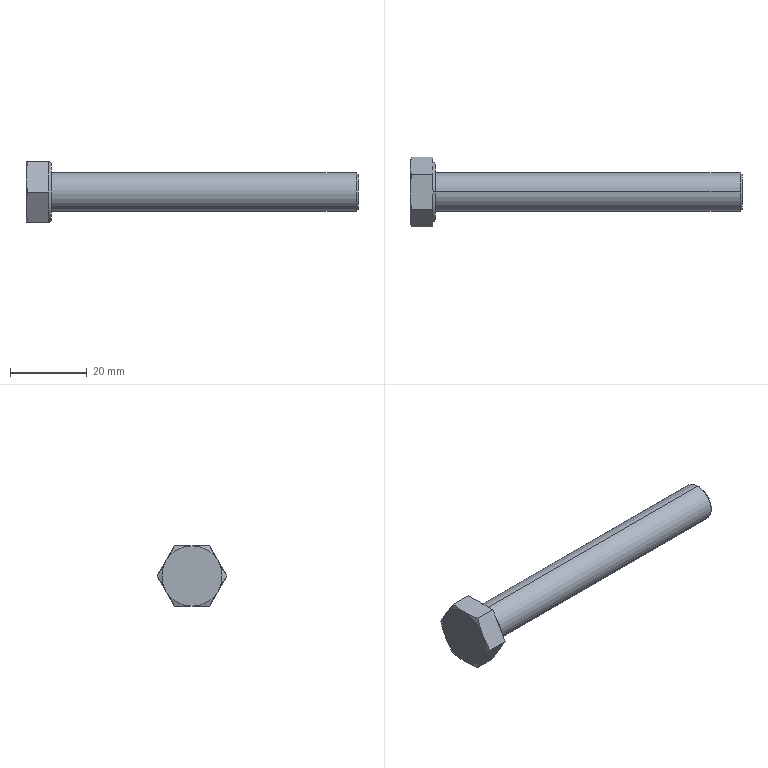Part | STEP file | hexagon head bolts-full thread_gb_GB_FASTENER_BOLT_STBAB A M10X80-N | 1 solid | 27 faces | box 86.58 x 18.163 x 15.73 mm | volume 7667 mm3 | plane 15 | cone 10 | cylinder 2 | commonest cylinder face diameters 10 x2